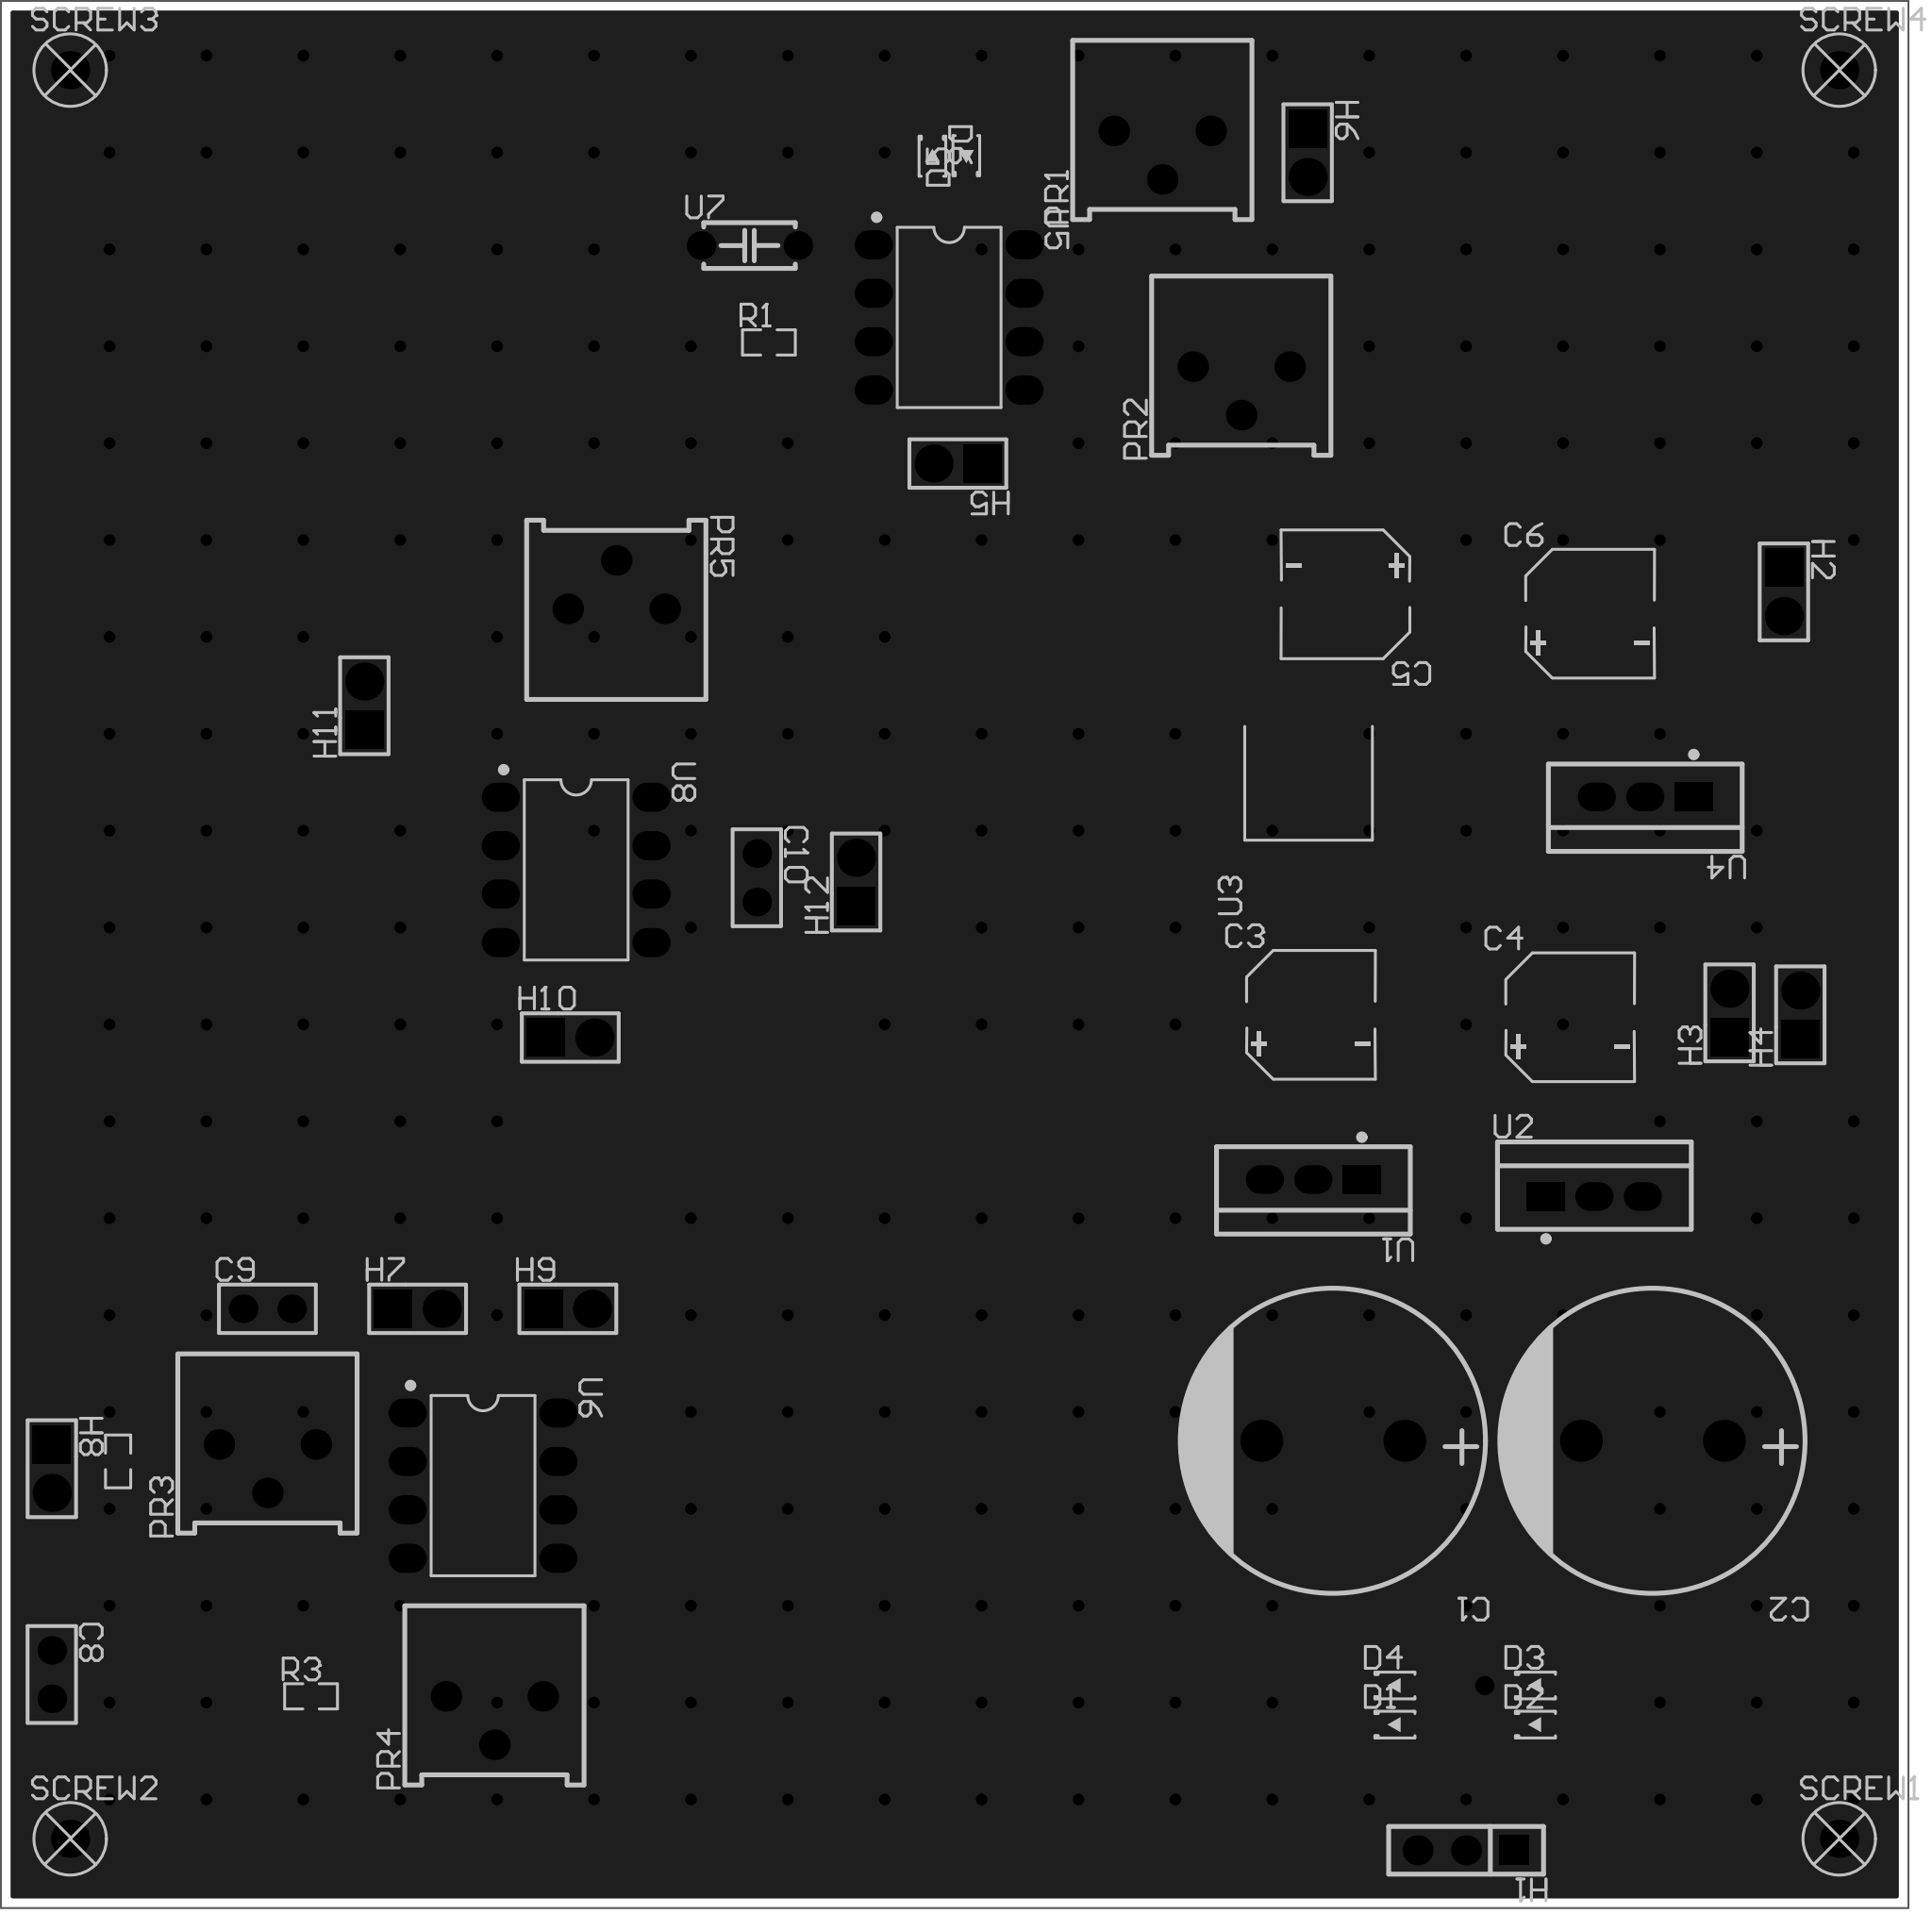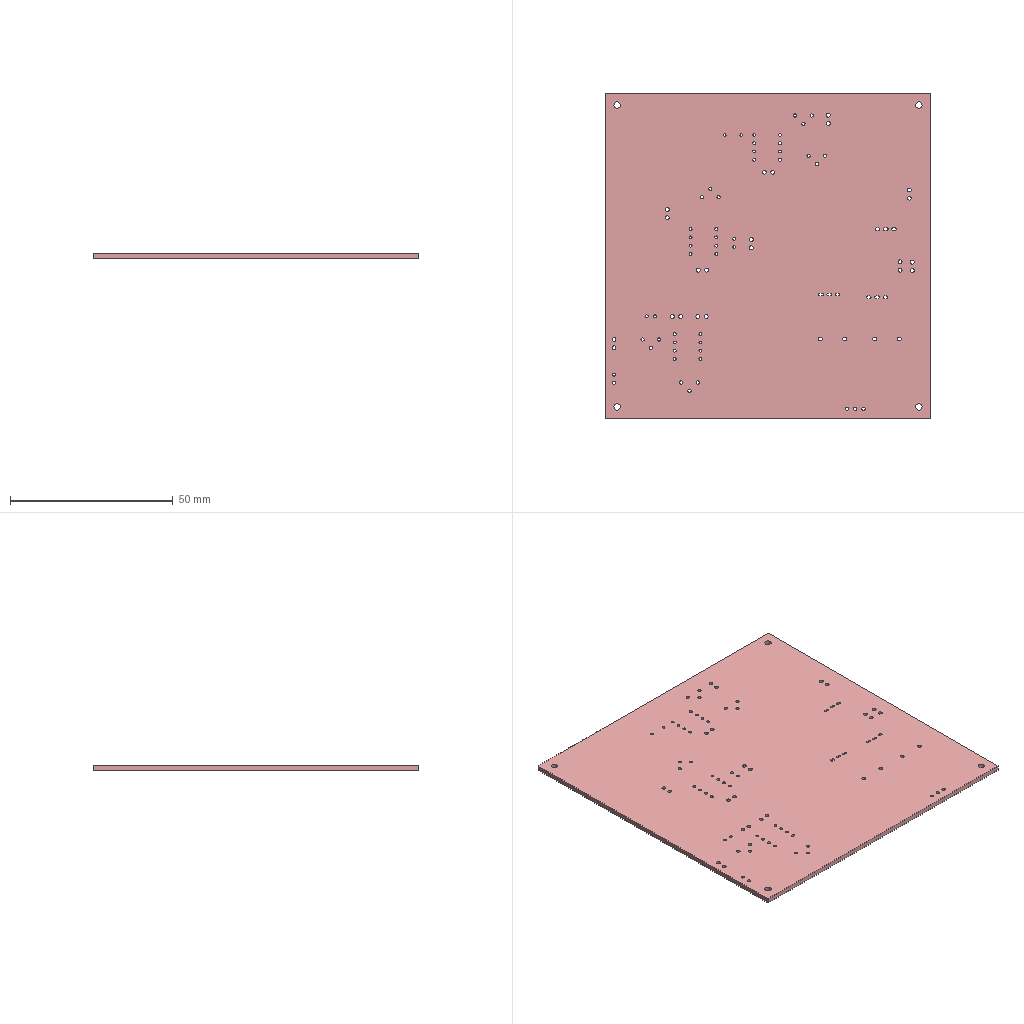Circuit board layout | Altium Designer | box 100 x 100 x 1.6 mm
Layer stack:
# Altium Designer layer stack of  (unit mm; dielectric type: 0 none, 1 core, 2 prepreg, 3 surface material)
index,name,kind,layer,copper_thickness_mm,dielectric_type,dielectric_thickness_mm,dielectric_material,dielectric_constant
0,Top Paste Mask Layer,other,,,,,,
1,Top Silkscreen Layer,other,,,,,,
2,Top Solder Mask Layer,dielectric,,,3,0.01,,3.3
3,Top Layer,copper,Top Layer,0.035,,,,
4,Dielectric1,dielectric,,,3,1.51,FR4,4.5
5,Bottom Layer,copper,Bottom Layer,0.035,,,,
6,Bottom Solder Mask Layer,dielectric,,,3,0.01,,3.3
7,Bottom Silkscreen Layer,other,,,,,,
8,Bottom Paste Mask Layer,other,,,,,,
# drill layer pairs: low layer,high layer
drill_pair,Top Layer,Bottom Layer
Part placement:
Designator,Comment,Layer,Footprint,Center-X(mm),Center-Y(mm),Rotation
C1,2200uF,TopLayer,CAP-TH_BD16.0-P7.50-D0.8-FD,161.901,114.112,180
C2,2200uF,TopLayer,CAP-TH_BD16.0-P7.50-D0.8-FD,178.655,114.112,180
C3,330uF,TopLayer,CAP-SMD_BD6.3-L6.6-W6.6-LS7.2-FD_3,160.753,136.446,0
C4,330uF,TopLayer,CAP-SMD_BD6.3-L6.6-W6.6-LS7.2-FD_3,174.342,136.319,0
C5,100uF,TopLayer,CAP-SMD_BD6.3-L6.6-W6.6-LS7.3-FD-H7.7,162.56,158.496,180
C6,100uF,TopLayer,CAP-SMD_BD6.3-L6.6-W6.6-LS7.3-FD-H7.7,175.387,157.48,0
C8,100nF,TopLayer,CAP-TH_L5.0-W2.5-P2.54-D0.7,94.742,101.854,270
C9,100nF,TopLayer,CAP-TH_L5.0-W2.5-P2.54-D0.7,106.045,121.035,0
C10,100nF,TopLayer,CAP-TH_L5.0-W2.5-P2.54-D0.7,131.704,143.632,270
D1,1N4007WS,TopLayer,SOD-323_L1.7-W1.3-LS2.5-RD,165.203,99.228,0
D2,1N4007WS,TopLayer,SOD-323_L1.7-W1.3-LS2.5-RD,172.569,99.228,0
D3,1N4007WS,TopLayer,SOD-323_L1.7-W1.3-LS2.5-RD,172.569,101.28,0
D4,1N4007WS,TopLayer,SOD-323_L1.7-W1.3-LS2.5-RD,165.203,101.28,0
D5,1N4007WS,TopLayer,SOD-323_L1.7-W1.3-LS2.5-RD,142.685,181.547,90
D6,1N4007WS,TopLayer,SOD-323_L1.7-W1.3-LS2.5-RD,140.906,181.419,270
H1,PM254V-11-03-H85,TopLayer,HDR-TH_3P-P2.54-V-F,168.886,92.638,180
H2,HX PH254-01-02-Z-L11.5 male header connector,TopLayer,HDR-TH_2P-P2.54-V-M,185.547,158.623,270
H3,HX PH254-01-02-Z-L11.5 male header connector,TopLayer,HDR-TH_2P-P2.54-V-M,182.696,136.549,90
H4,HX PH254-01-02-Z-L11.5 male header connector,TopLayer,HDR-TH_2P-P2.54-V-M,186.407,136.446,90
H5,HX PH254-01-02-Z-L11.5 male header connector,TopLayer,HDR-TH_2P-P2.54-V-M,142.24,165.354,180
H6,HX PH254-01-02-Z-L11.5 male header connector,TopLayer,HDR-TH_2P-P2.54-V-M,160.579,181.65,270
H7,HX PH254-01-02-Z-L11.5 male header connector,TopLayer,HDR-TH_2P-P2.54-V-M,113.917,121.031,0
H8,HX PH254-01-02-Z-L11.5 male header connector,TopLayer,HDR-TH_2P-P2.54-V-M,94.742,112.649,270
H9,HX PH254-01-02-Z-L11.5 male header connector,TopLayer,HDR-TH_2P-P2.54-V-M,121.793,121.031,0
H10,HX PH254-01-02-Z-L11.5 male header connector,TopLayer,HDR-TH_2P-P2.54-V-M,121.92,135.255,0
H11,HX PH254-01-02-Z-L11.5 male header connector,TopLayer,HDR-TH_2P-P2.54-V-M,111.125,152.654,90
H12,HX PH254-01-02-Z-L11.5 male header connector,TopLayer,HDR-TH_2P-P2.54-V-M,136.906,143.412,90
PR1,5K,TopLayer,R_3386P,152.959,181.524,90
PR2,5K,TopLayer,R_3386P,157.099,169.164,90
PR3,1K,TopLayer,R_3386P,106.045,112.649,90
PR4,1K,TopLayer,R_3386P,117.945,99.441,90
PR5,2K,TopLayer,R_3386P,124.333,159.004,270
R1,1kΩ,TopLayer,R0603,132.334,171.704,0
R2,1kΩ,TopLayer,R0603,98.216,113.03,270
R3,1kΩ,TopLayer,R0603,108.331,100.711,0
SCREW1,,TopLayer,M2螺丝,188.446,93.24,0
SCREW2,,TopLayer,M2螺丝,95.704,93.24,0
SCREW3,,TopLayer,M2螺丝,95.704,185.982,0
SCREW4,,TopLayer,M2螺丝,188.446,185.982,0
U1,LM7812CT/NOPB,TopLayer,TO-220-3_L10.2-W4.6-P2.54-L,160.88,127.81,180
U2,LM7912CT/NOPB,TopLayer,TO-220-3_L10.2-W4.6-P2.54-L,175.612,126.922,0
U3,LM7805-5V,TopLayer,TO-252-2_L6.6-W6.1-P4.58-LS9.9-TL,160.626,146.988,90
U4,LM7812CT/NOPB,TopLayer,TO-220-3_L10.2-W4.6-P2.54-L,178.279,147.876,180
U5,LF411CP,TopLayer,PDIP-8_L9.3-W6.4-P2.54-LS7.9-BL-1,141.783,173.014,270
U6,LF411CP,TopLayer,PDIP-8_L9.3-W6.4-P2.54-LS7.9-BL-1,117.348,111.76,270
U7,470nF,TopLayer,CAP-TH_L4.8-W2.4-P5.08-D0.6,131.318,176.784,0
U8,LF411CP,TopLayer,PDIP-8_L9.3-W6.4-P2.54-LS7.9-BL-1,122.231,144.047,270
Pad and via stacks:
# Altium Designer via and pad stacks of  (unit mm). Each distinct definition once, with the count of objects using it.
# via: kind,start_layer,end_layer,hole_mm,diameter_mm,mode(0 simple;1 top-mid-bottom;2 full stack),diameter_per_layer,count,example_net
# pad: kind,layer,hole_mm,hole_type(0 round;1 square;2 slot),plating,top_size,top_shape(1 round;2 rect;3 octagon;9 rounded rect),mid_size,bottom_size,mode,footprint,size_per_layer,count,example
pad,Multi-Layer,1.2,0,plated,2.2x2.2,1,2.2x2.2,2.2x2.2,0,CAP-TH_BD16.0-P7.50-D0.8-FD,,4,C1.1
pad,Multi-Layer,0.9,0,plated,1.5x1.5,1,1.5x1.5,1.5x1.5,0,CAP-TH_L5.0-W2.5-P2.54-D0.7,,6,C8.1
pad,Multi-Layer,1.02,0,plated,1.575x1.575,1,1.575x1.575,1.575x1.575,0,HDR-TH_3P-P2.54-V-F,,2,H1.3
pad,Multi-Layer,1.02,0,plated,1.575x1.575,2,1.575x1.575,1.575x1.575,0,HDR-TH_3P-P2.54-V-F,,1,H1.1
pad,Multi-Layer,1.2,0,plated,2x2,2,2x2,2x2,0,HDR-TH_2P-P2.54-V-M,,11,H2.1
pad,Multi-Layer,1.2,0,plated,2x2,1,2x2,2x2,0,HDR-TH_2P-P2.54-V-M,,11,H2.2
pad,Multi-Layer,1.001,0,plated,1.6x1.6,1,1.6x1.6,1.6x1.6,0,R_3386P,,15,PR1.2
pad,Multi-Layer,2,0,plated,2x2,1,2x2,2x2,0,M2\u00C2\u00DD\u00CB\u00BF,,4,SCREW1.1
pad,Multi-Layer,0.8,2,plated,2x1.5,1,2x1.5,2x1.5,0,TO-220-3_L10.2-W4.6-P2.54-L,,6,U1.2
pad,Multi-Layer,0.8,2,plated,2x1.5,2,2x1.5,2x1.5,0,TO-220-3_L10.2-W4.6-P2.54-L,,3,U1.1
pad,Multi-Layer,0.9,0,plated,1.524x2,1,1.524x2,1.524x2,0,PDIP-8_L9.3-W6.4-P2.54-LS7.9-BL-1,,24,U5.1
pad,Multi-Layer,0.8,0,plated,1.5x1.5,1,1.5x1.5,1.5x1.5,0,CAP-TH_L4.8-W2.4-P5.08-D0.6,,2,U7.2
pad,Top Layer,0,0,plated,3.5x1.2,2,3.5x1.2,3.5x1.2,0,CAP-SMD_BD6.3-L6.6-W6.6-LS7.2-FD_3,,4,C3.2
pad,Top Layer,0,0,plated,3.5x1.2,2,3.5x1.2,3.5x1.2,0,CAP-SMD_BD6.3-L6.6-W6.6-LS7.3-FD-H7.7,,4,C5.1
pad,Top Layer,0,0,plated,0.8x0.8,2,0.8x0.8,0.8x0.8,0,SOD-323_L1.7-W1.3-LS2.5-RD,,12,D1.1
pad,Top Layer,0,0,plated,0.8065x0.864,2,0.8065x0.864,0.8065x0.864,0,R0603,,6,R1.2
pad,Top Layer,0,0,plated,2.409x0.9786,2,2.409x0.9786,2.409x0.9786,0,TO-252-2_L6.6-W6.1-P4.58-LS9.9-TL,,2,U3.1
pad,Top Layer,0,0,plated,5.711x5.548,2,5.711x5.548,5.711x5.548,0,TO-252-2_L6.6-W6.1-P4.58-LS9.9-TL,,1,U3.2
via,Top Layer,Bottom Layer,0.5004,1,0,,1,$1N35
via,Top Layer,Bottom Layer,0.3048,0.6096,0,,275,GND
Copper pours:
name,layer,net,type(0 solid;1 hatched;2 none)
Top Layer-GND,Top Layer,GND,0
Bottom Layer-GND,Bottom Layer,GND,0
Design rules, without the lines most boards share:
# Altium Designer design rules of  (exported by Altium Designer, unit mm)
# columns: name | kind | enabled | priority | scope1 | scope2 | descriptor | typed fields (field=value)
copperThickness2oz | 0 | disabled | 1 | All | All | Clearance Constraint (Gap=6mil) (Disabled)(All),(All) | gap=0.1524
Copper_copperRegion | 0 | disabled | 2 | All | All | Clearance Constraint (Gap=8mil) (Disabled)(All),(All) | gap=0.2032
Copper_copperRegion_1 | 63 | disabled | 2 | All | All | Board Clearance Constraint (Gap=0mil) (Disabled)(All) |
Plane_innerPlane | 0 | disabled | 3 | All | All | Clearance Constraint (Gap=8mil) (Disabled)(All),(All) | gap=0.2032
Plane_innerPlane_1 | 63 | disabled | 3 | All | All | Board Clearance Constraint (Gap=0mil) (Disabled)(All) |
copperThickness1oz | 0 | enabled | 4 | All | All | Clearance Constraint (Gap=8mil) (All),(All) | gap=0.2032
otherClearance | 52 | enabled | 1 | All | All | Hole To Hole Clearance (Gap=11.8mil) (All),(All) | gap=0.2997
copperThickness2oz_2 | 2 | enabled | 1 | (InNet('-5V') OR InNet('-12V') OR InNet('+5V') OR InNet('+12V')) | All | Width Constraint (Min=8mil) (Max=100mil) (Preferred=10mil) ((InNet('-5V') OR InNet('-12V') OR InNet('+5V') OR InNet('+12V'))) |
VCC and GND | 2 | disabled | 2 | All | All | Width Constraint (Min=10mil) (Max=30mil) (Preferred=30mil) (Disabled)(All) |
copperThickness1oz_2 | 2 | enabled | 3 | All | All | Width Constraint (Min=8mil) (Max=50mil) (Preferred=50mil) (All) |
viaSize | 11 | enabled | 1 | All | All | Routing Via (MinHoleWidth=11.8mil) (MaxHoleWidth=248mil) (PreferredHoleWidth=12mil) (MinWidth=19.7mil) (MaxWidth=393.7mil) (PreferedWidth=24mil) (All) | via_min_hole=0.2997 via_max_hole=6.299 via_preferred_diameter=0.6096 via_preferred_hole=0.3048